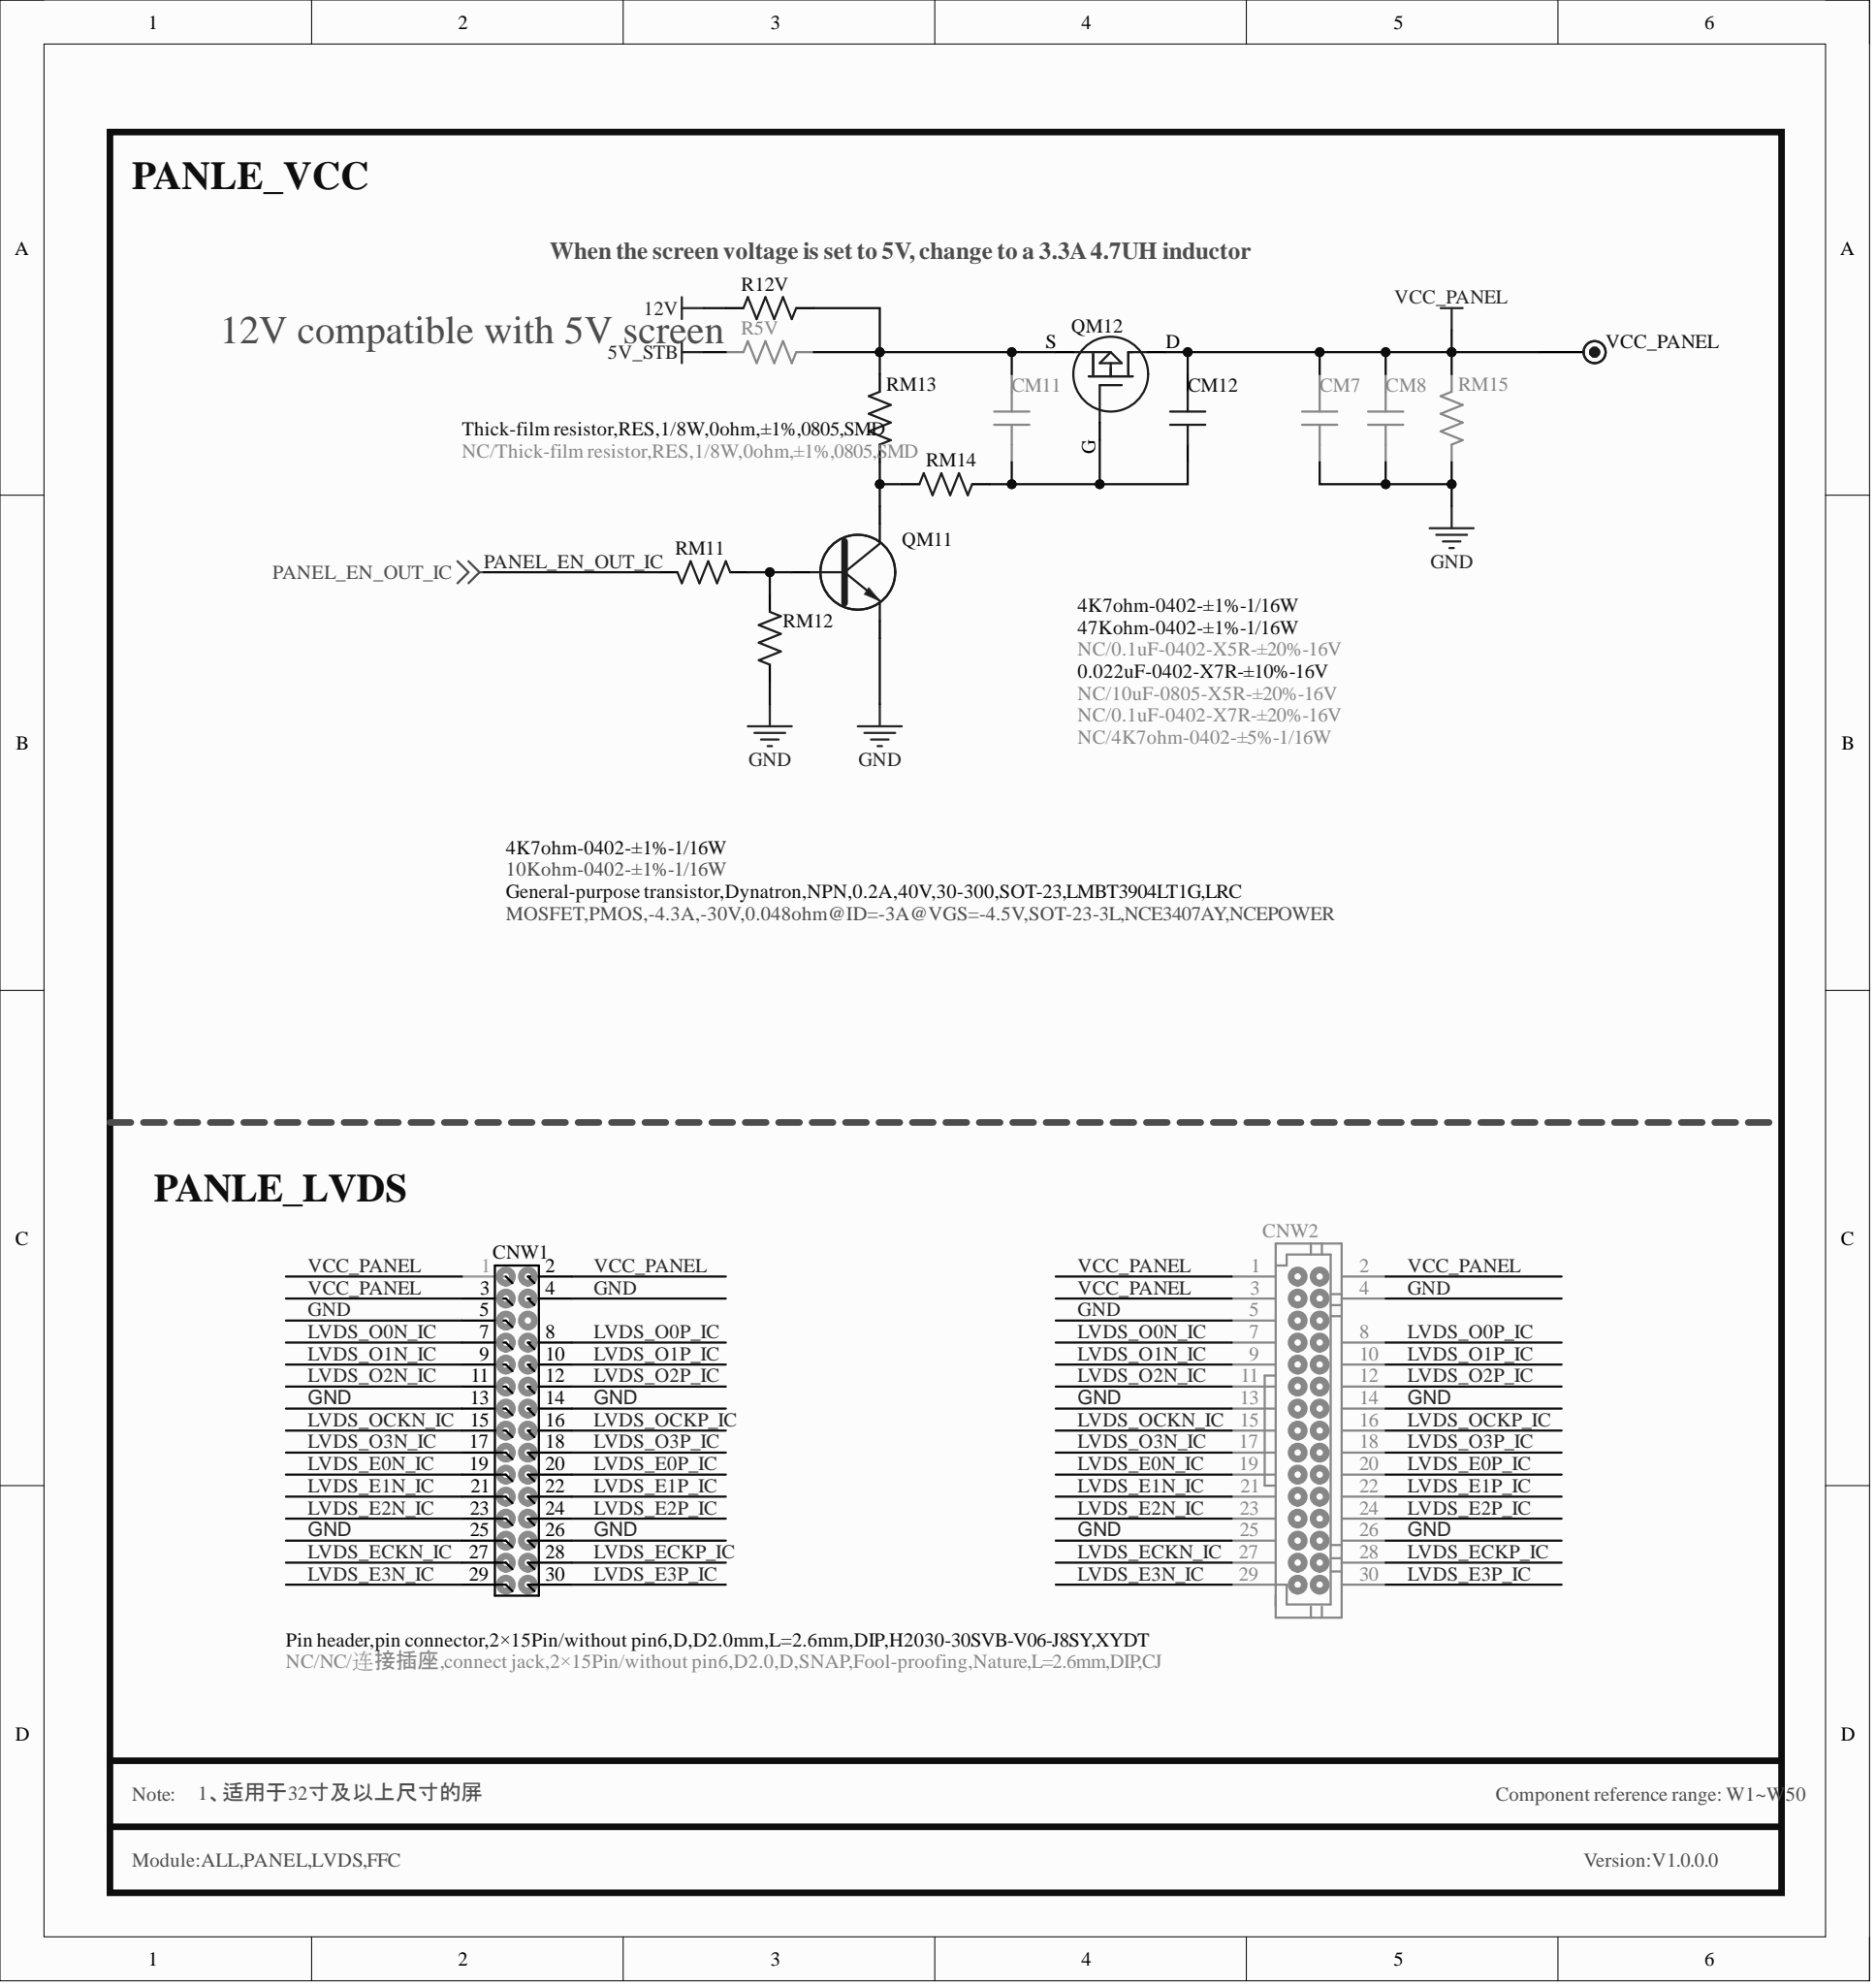Circuit board | Altium Designer | 527 parts | 243 nets | one sheet of the schematic
Parts on this sheet (reference | value | footprint):
CM7 | NC/10uF-0805-X5R-±20%-16V | C0805
CM8 | NC/0.1uF-0402-X7R-±20%-16V | C0402
CM11 | NC/0.1uF-0402-X5R-±20%-16V | C0402
CM12 | 0.022uF-0402-X7R-±10%-16V | C0402
CNW1 | Pin header,pin connector,2×15Pin/without pin6,D,D2.0mm,L=2.6mm,DIP,H2030-30SVB-V06-J8SY,XYDT | SIP2*15/2.0D-2
CNW2 | NC/NC/连接插座,connect jack,2×15Pin/without pin6,D2.0,D,SNAP,Fool-proofing,Nature,L=2.6mm,DIP,CJ | SIP2*15/2.0D-11
QM11 | General-purpose transistor,Dynatron,NPN,0.2A,40V,30-300,SOT-23,LMBT3904LT1G,LRC | SOT-23
QM12 | MOSFET,PMOS,-4.3A,-30V,0.048ohm@ID=-3A@VGS=-4.5V,SOT-23-3L,NCE3407AY,NCEPOWER | SOT-23-1
R5V | NC/Thick-film resistor,RES,1/8W,0ohm,±1%,0805,SMD | R0805
R12V | Thick-film resistor,RES,1/8W,0ohm,±1%,0805,SMD | R0805
RM11 | 4K7ohm-0402-±1%-1/16W | R0402
RM12 | 10Kohm-0402-±1%-1/16W | R0402
RM13 | 4K7ohm-0402-±1%-1/16W | R0402
RM14 | 47Kohm-0402-±1%-1/16W | R0402
RM15 | NC/4K7ohm-0402-±5%-1/16W | R0402
VCC_PANEL | TEST | TP
Nets of these parts (net: part-pin ...):
VCC_PANEL: CM7-1 CM8-2 CM12-1 QM12-D RM15-1 VCC_PANEL-1 CNW1-1 CNW1-2 CNW1-3 CNW2-1 CNW2-2 CNW2-3
PANEL_EN_OUT_IC: RM11-1
NetQM11_C: QM11-C RM13-2 RM14-1
NetQM11_B: QM11-B RM11-2 RM12-1
NetCM11_2: CM11-2 QM12-S R5V-2 R12V-2 RM13-1
NetCM11_1: CM11-1 CM12-2 QM12-G RM14-2
LVDS_OCKP_IC: CNW1-16 CNW2-16
LVDS_OCKN_IC: CNW1-15 CNW2-15
LVDS_O3P_IC: CNW1-18 CNW2-18
LVDS_O3N_IC: CNW1-17 CNW2-17
LVDS_O2P_IC: CNW1-12 CNW2-12
LVDS_O2N_IC: CNW1-11 CNW2-11
LVDS_O1P_IC: CNW1-10 CNW2-10
LVDS_O1N_IC: CNW1-9 CNW2-9
LVDS_O0P_IC: CNW1-8 CNW2-8
LVDS_O0N_IC: CNW1-7 CNW2-7
LVDS_ECKP_IC: CNW1-28 CNW2-28
LVDS_ECKN_IC: CNW1-27 CNW2-27
LVDS_E3P_IC: CNW1-30 CNW2-30
LVDS_E3N_IC: CNW1-29 CNW2-29
LVDS_E2P_IC: CNW1-24 CNW2-24
LVDS_E2N_IC: CNW1-23 CNW2-23
LVDS_E1P_IC: CNW1-22 CNW2-22
LVDS_E1N_IC: CNW1-21 CNW2-21
LVDS_E0P_IC: CNW1-20 CNW2-20
LVDS_E0N_IC: CNW1-19 CNW2-19
GND: CM7-2 CM8-1 QM11-E RM12-2 RM15-2 CNW1-4 CNW1-5 CNW1-13 CNW1-14 CNW1-25 CNW1-26 CNW2-4 CNW2-5 CNW2-13 CNW2-14 CNW2-25 CNW2-26
12V: R12V-1
5V_STB: R5V-1